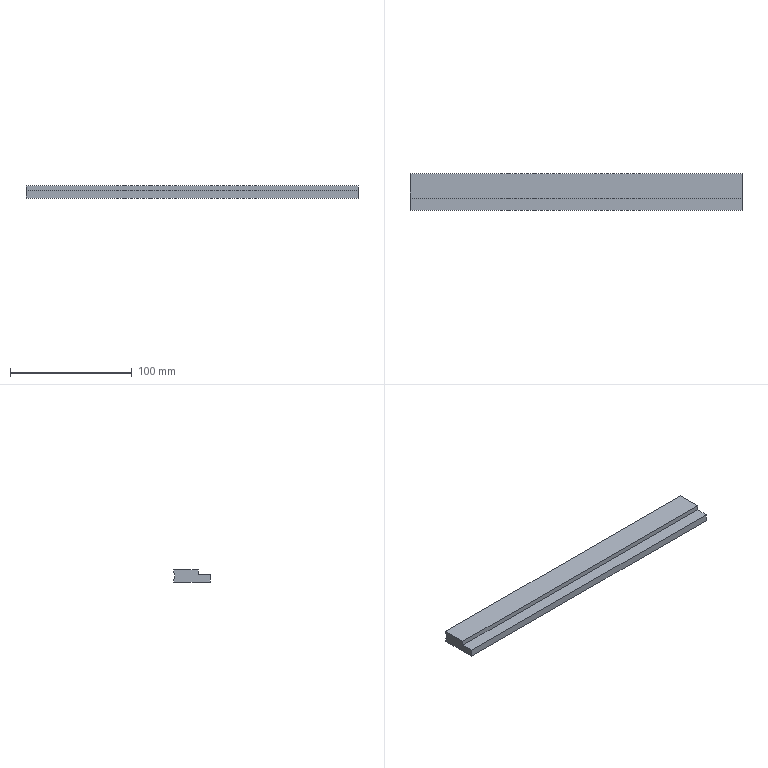Part | STEP file | 001-011-Blanking flip guide rod mounting seat | 1 solid | 10 faces | box 273 x 30 x 10 mm | volume 69990 mm3 | plane 9 | cylinder 1 | commonest cylinder face diameters 8 x1
STEP:
#1=CARTESIAN_POINT('',(0.,0.,0.));
#2=DIRECTION('',(0.,0.,1.));
#3=DIRECTION('',(1.,0.,0.));
#4=AXIS2_PLACEMENT_3D('',#1,#2,#3);
#5=CARTESIAN_POINT('',(-136.5,15.,2.354));
#6=VERTEX_POINT('',#5);
#7=CARTESIAN_POINT('',(-136.5,15.,0.));
#8=VERTEX_POINT('',#7);
#9=CARTESIAN_POINT('',(-136.5,15.,10.));
#10=DIRECTION('',(0.,0.,-1.));
#11=VECTOR('',#10,1.);
#12=LINE('',#9,#11);
#13=CARTESIAN_POINT('',(-136.5,15.,10.));
#14=DIRECTION('',(0.,-1.,0.));
#15=DIRECTION('',(1.,0.,0.));
#16=AXIS2_PLACEMENT_3D('',#13,#14,#15);
#17=PLANE('',#16);
#18=CARTESIAN_POINT('',(0.,0.));
#19=DIRECTION('',(0.,-1.));
#20=VECTOR('',#19,1.);
#21=LINE('',#18,#20);
#22=(GEOMETRIC_REPRESENTATION_CONTEXT(2)PARAMETRIC_REPRESENTATION_CONTEXT()REPRESENTATION_CONTEXT('',''));
#23=DEFINITIONAL_REPRESENTATION('',(#21),#22);
#24=PCURVE('',#17,#23);
#25=CARTESIAN_POINT('',(-136.5,-15.,10.));
#26=DIRECTION('',(1.,0.,0.));
#27=DIRECTION('',(0.,0.,-1.));
#28=AXIS2_PLACEMENT_3D('',#25,#26,#27);
#29=PLANE('',#28);
#30=CARTESIAN_POINT('',(0.,30.));
#31=DIRECTION('',(1.,0.));
#32=VECTOR('',#31,1.);
#33=LINE('',#30,#32);
#34=(GEOMETRIC_REPRESENTATION_CONTEXT(2)PARAMETRIC_REPRESENTATION_CONTEXT()REPRESENTATION_CONTEXT('',''));
#35=DEFINITIONAL_REPRESENTATION('',(#33),#34);
#36=PCURVE('',#29,#35);
#37=SURFACE_CURVE('',#12,(#24,#36),.PCURVE_S1.);
#38=EDGE_CURVE('',#6,#8,#37,.T.);
#39=ORIENTED_EDGE('',*,*,#38,.F.);
#40=CARTESIAN_POINT('',(136.5,15.,2.354));
#41=VERTEX_POINT('',#40);
#42=CARTESIAN_POINT('',(-136.5,15.,2.354));
#43=DIRECTION('',(1.,0.,0.));
#44=VECTOR('',#43,1.);
#45=LINE('',#42,#44);
#46=CARTESIAN_POINT('',(0.,-7.646));
#47=DIRECTION('',(1.,0.));
#48=VECTOR('',#47,1.);
#49=LINE('',#46,#48);
#50=(GEOMETRIC_REPRESENTATION_CONTEXT(2)PARAMETRIC_REPRESENTATION_CONTEXT()REPRESENTATION_CONTEXT('',''));
#51=DEFINITIONAL_REPRESENTATION('',(#49),#50);
#52=PCURVE('',#17,#51);
#53=CARTESIAN_POINT('',(-136.5,18.,5.));
#54=DIRECTION('',(1.,0.,0.));
#55=DIRECTION('',(0.,0.,-1.));
#56=AXIS2_PLACEMENT_3D('',#53,#54,#55);
#57=CYLINDRICAL_SURFACE('',#56,4.);
#58=CARTESIAN_POINT('',(5.435,0.));
#59=DIRECTION('',(0.,1.));
#60=VECTOR('',#59,1.);
#61=LINE('',#58,#60);
#62=(GEOMETRIC_REPRESENTATION_CONTEXT(2)PARAMETRIC_REPRESENTATION_CONTEXT()REPRESENTATION_CONTEXT('',''));
#63=DEFINITIONAL_REPRESENTATION('',(#61),#62);
#64=PCURVE('',#57,#63);
#65=SURFACE_CURVE('',#45,(#52,#64),.PCURVE_S1.);
#66=EDGE_CURVE('',#6,#41,#65,.T.);
#67=ORIENTED_EDGE('',*,*,#66,.T.);
#68=CARTESIAN_POINT('',(136.5,15.,0.));
#69=VERTEX_POINT('',#68);
#70=CARTESIAN_POINT('',(136.5,15.,10.));
#71=DIRECTION('',(0.,0.,-1.));
#72=VECTOR('',#71,1.);
#73=LINE('',#70,#72);
#74=CARTESIAN_POINT('',(273.,0.));
#75=DIRECTION('',(0.,-1.));
#76=VECTOR('',#75,1.);
#77=LINE('',#74,#76);
#78=(GEOMETRIC_REPRESENTATION_CONTEXT(2)PARAMETRIC_REPRESENTATION_CONTEXT()REPRESENTATION_CONTEXT('',''));
#79=DEFINITIONAL_REPRESENTATION('',(#77),#78);
#80=PCURVE('',#17,#79);
#81=CARTESIAN_POINT('',(136.5,-15.,10.));
#82=DIRECTION('',(-1.,0.,0.));
#83=DIRECTION('',(0.,0.,1.));
#84=AXIS2_PLACEMENT_3D('',#81,#82,#83);
#85=PLANE('',#84);
#86=CARTESIAN_POINT('',(0.,30.));
#87=DIRECTION('',(-1.,0.));
#88=VECTOR('',#87,1.);
#89=LINE('',#86,#88);
#90=(GEOMETRIC_REPRESENTATION_CONTEXT(2)PARAMETRIC_REPRESENTATION_CONTEXT()REPRESENTATION_CONTEXT('',''));
#91=DEFINITIONAL_REPRESENTATION('',(#89),#90);
#92=PCURVE('',#85,#91);
#93=SURFACE_CURVE('',#73,(#80,#92),.PCURVE_S1.);
#94=EDGE_CURVE('',#41,#69,#93,.T.);
#95=ORIENTED_EDGE('',*,*,#94,.T.);
#96=CARTESIAN_POINT('',(-136.5,15.,0.));
#97=DIRECTION('',(-1.,0.,0.));
#98=VECTOR('',#97,1.);
#99=LINE('',#96,#98);
#100=CARTESIAN_POINT('',(0.,-10.));
#101=DIRECTION('',(-1.,0.));
#102=VECTOR('',#101,1.);
#103=LINE('',#100,#102);
#104=(GEOMETRIC_REPRESENTATION_CONTEXT(2)PARAMETRIC_REPRESENTATION_CONTEXT()REPRESENTATION_CONTEXT('',''));
#105=DEFINITIONAL_REPRESENTATION('',(#103),#104);
#106=PCURVE('',#17,#105);
#107=CARTESIAN_POINT('',(0.,0.,0.));
#108=DIRECTION('',(0.,0.,-1.));
#109=DIRECTION('',(-1.,0.,0.));
#110=AXIS2_PLACEMENT_3D('',#107,#108,#109);
#111=PLANE('',#110);
#112=CARTESIAN_POINT('',(136.5,15.));
#113=DIRECTION('',(1.,0.));
#114=VECTOR('',#113,1.);
#115=LINE('',#112,#114);
#116=(GEOMETRIC_REPRESENTATION_CONTEXT(2)PARAMETRIC_REPRESENTATION_CONTEXT()REPRESENTATION_CONTEXT('',''));
#117=DEFINITIONAL_REPRESENTATION('',(#115),#116);
#118=PCURVE('',#111,#117);
#119=SURFACE_CURVE('',#99,(#106,#118),.PCURVE_S1.);
#120=EDGE_CURVE('',#69,#8,#119,.T.);
#121=ORIENTED_EDGE('',*,*,#120,.T.);
#122=EDGE_LOOP('',(#39,#67,#95,#121));
#123=FACE_BOUND('',#122,.T.);
#124=ADVANCED_FACE('',(#123),#17,.F.);
#125=CARTESIAN_POINT('',(136.5,-5.,10.));
#126=VERTEX_POINT('',#125);
#127=CARTESIAN_POINT('',(136.5,15.,10.));
#128=VERTEX_POINT('',#127);
#129=CARTESIAN_POINT('',(136.5,-15.,10.));
#130=DIRECTION('',(0.,1.,0.));
#131=VECTOR('',#130,1.);
#132=LINE('',#129,#131);
#133=CARTESIAN_POINT('',(0.,0.));
#134=DIRECTION('',(0.,1.));
#135=VECTOR('',#134,1.);
#136=LINE('',#133,#135);
#137=(GEOMETRIC_REPRESENTATION_CONTEXT(2)PARAMETRIC_REPRESENTATION_CONTEXT()REPRESENTATION_CONTEXT('',''));
#138=DEFINITIONAL_REPRESENTATION('',(#136),#137);
#139=PCURVE('',#85,#138);
#140=CARTESIAN_POINT('',(0.,0.,10.));
#141=DIRECTION('',(0.,0.,-1.));
#142=DIRECTION('',(-1.,0.,0.));
#143=AXIS2_PLACEMENT_3D('',#140,#141,#142);
#144=PLANE('',#143);
#145=CARTESIAN_POINT('',(-136.5,-15.));
#146=DIRECTION('',(0.,1.));
#147=VECTOR('',#146,1.);
#148=LINE('',#145,#147);
#149=(GEOMETRIC_REPRESENTATION_CONTEXT(2)PARAMETRIC_REPRESENTATION_CONTEXT()REPRESENTATION_CONTEXT('',''));
#150=DEFINITIONAL_REPRESENTATION('',(#148),#149);
#151=PCURVE('',#144,#150);
#152=SURFACE_CURVE('',#132,(#139,#151),.PCURVE_S1.);
#153=EDGE_CURVE('',#126,#128,#152,.T.);
#154=ORIENTED_EDGE('',*,*,#153,.F.);
#155=CARTESIAN_POINT('',(136.5,-5.,6.));
#156=VERTEX_POINT('',#155);
#157=CARTESIAN_POINT('',(136.5,-5.,6.));
#158=DIRECTION('',(0.,0.,1.));
#159=VECTOR('',#158,1.);
#160=LINE('',#157,#159);
#161=CARTESIAN_POINT('',(-4.,10.));
#162=DIRECTION('',(1.,0.));
#163=VECTOR('',#162,1.);
#164=LINE('',#161,#163);
#165=(GEOMETRIC_REPRESENTATION_CONTEXT(2)PARAMETRIC_REPRESENTATION_CONTEXT()REPRESENTATION_CONTEXT('',''));
#166=DEFINITIONAL_REPRESENTATION('',(#164),#165);
#167=PCURVE('',#85,#166);
#168=CARTESIAN_POINT('',(-136.5,-5.,6.));
#169=DIRECTION('',(0.,1.,0.));
#170=DIRECTION('',(0.,0.,1.));
#171=AXIS2_PLACEMENT_3D('',#168,#169,#170);
#172=PLANE('',#171);
#173=CARTESIAN_POINT('',(0.,273.));
#174=DIRECTION('',(1.,0.));
#175=VECTOR('',#174,1.);
#176=LINE('',#173,#175);
#177=(GEOMETRIC_REPRESENTATION_CONTEXT(2)PARAMETRIC_REPRESENTATION_CONTEXT()REPRESENTATION_CONTEXT('',''));
#178=DEFINITIONAL_REPRESENTATION('',(#176),#177);
#179=PCURVE('',#172,#178);
#180=SURFACE_CURVE('',#160,(#167,#179),.PCURVE_S1.);
#181=EDGE_CURVE('',#156,#126,#180,.T.);
#182=ORIENTED_EDGE('',*,*,#181,.F.);
#183=CARTESIAN_POINT('',(136.5,-15.,6.));
#184=VERTEX_POINT('',#183);
#185=CARTESIAN_POINT('',(136.5,-15.,6.));
#186=DIRECTION('',(0.,1.,0.));
#187=VECTOR('',#186,1.);
#188=LINE('',#185,#187);
#189=CARTESIAN_POINT('',(-4.,0.));
#190=DIRECTION('',(0.,1.));
#191=VECTOR('',#190,1.);
#192=LINE('',#189,#191);
#193=(GEOMETRIC_REPRESENTATION_CONTEXT(2)PARAMETRIC_REPRESENTATION_CONTEXT()REPRESENTATION_CONTEXT('',''));
#194=DEFINITIONAL_REPRESENTATION('',(#192),#193);
#195=PCURVE('',#85,#194);
#196=CARTESIAN_POINT('',(0.,0.,6.));
#197=DIRECTION('',(0.,0.,-1.));
#198=DIRECTION('',(-1.,0.,0.));
#199=AXIS2_PLACEMENT_3D('',#196,#197,#198);
#200=PLANE('',#199);
#201=CARTESIAN_POINT('',(-136.5,-15.));
#202=DIRECTION('',(0.,1.));
#203=VECTOR('',#202,1.);
#204=LINE('',#201,#203);
#205=(GEOMETRIC_REPRESENTATION_CONTEXT(2)PARAMETRIC_REPRESENTATION_CONTEXT()REPRESENTATION_CONTEXT('',''));
#206=DEFINITIONAL_REPRESENTATION('',(#204),#205);
#207=PCURVE('',#200,#206);
#208=SURFACE_CURVE('',#188,(#195,#207),.PCURVE_S1.);
#209=EDGE_CURVE('',#184,#156,#208,.T.);
#210=ORIENTED_EDGE('',*,*,#209,.F.);
#211=CARTESIAN_POINT('',(136.5,-15.,0.));
#212=VERTEX_POINT('',#211);
#213=CARTESIAN_POINT('',(136.5,-15.,10.));
#214=DIRECTION('',(0.,0.,-1.));
#215=VECTOR('',#214,1.);
#216=LINE('',#213,#215);
#217=CARTESIAN_POINT('',(0.,0.));
#218=DIRECTION('',(-1.,0.));
#219=VECTOR('',#218,1.);
#220=LINE('',#217,#219);
#221=(GEOMETRIC_REPRESENTATION_CONTEXT(2)PARAMETRIC_REPRESENTATION_CONTEXT()REPRESENTATION_CONTEXT('',''));
#222=DEFINITIONAL_REPRESENTATION('',(#220),#221);
#223=PCURVE('',#85,#222);
#224=CARTESIAN_POINT('',(-136.5,-15.,10.));
#225=DIRECTION('',(0.,1.,0.));
#226=DIRECTION('',(-1.,0.,0.));
#227=AXIS2_PLACEMENT_3D('',#224,#225,#226);
#228=PLANE('',#227);
#229=CARTESIAN_POINT('',(-273.,0.));
#230=DIRECTION('',(0.,-1.));
#231=VECTOR('',#230,1.);
#232=LINE('',#229,#231);
#233=(GEOMETRIC_REPRESENTATION_CONTEXT(2)PARAMETRIC_REPRESENTATION_CONTEXT()REPRESENTATION_CONTEXT('',''));
#234=DEFINITIONAL_REPRESENTATION('',(#232),#233);
#235=PCURVE('',#228,#234);
#236=SURFACE_CURVE('',#216,(#223,#235),.PCURVE_S1.);
#237=EDGE_CURVE('',#184,#212,#236,.T.);
#238=ORIENTED_EDGE('',*,*,#237,.T.);
#239=CARTESIAN_POINT('',(136.5,-15.,0.));
#240=DIRECTION('',(0.,1.,0.));
#241=VECTOR('',#240,1.);
#242=LINE('',#239,#241);
#243=CARTESIAN_POINT('',(-10.,0.));
#244=DIRECTION('',(0.,1.));
#245=VECTOR('',#244,1.);
#246=LINE('',#243,#245);
#247=(GEOMETRIC_REPRESENTATION_CONTEXT(2)PARAMETRIC_REPRESENTATION_CONTEXT()REPRESENTATION_CONTEXT('',''));
#248=DEFINITIONAL_REPRESENTATION('',(#246),#247);
#249=PCURVE('',#85,#248);
#250=CARTESIAN_POINT('',(-136.5,-15.));
#251=DIRECTION('',(0.,1.));
#252=VECTOR('',#251,1.);
#253=LINE('',#250,#252);
#254=(GEOMETRIC_REPRESENTATION_CONTEXT(2)PARAMETRIC_REPRESENTATION_CONTEXT()REPRESENTATION_CONTEXT('',''));
#255=DEFINITIONAL_REPRESENTATION('',(#253),#254);
#256=PCURVE('',#111,#255);
#257=SURFACE_CURVE('',#242,(#249,#256),.PCURVE_S1.);
#258=EDGE_CURVE('',#212,#69,#257,.T.);
#259=ORIENTED_EDGE('',*,*,#258,.T.);
#260=ORIENTED_EDGE('',*,*,#94,.F.);
#261=CARTESIAN_POINT('',(136.5,15.,7.646));
#262=VERTEX_POINT('',#261);
#263=CARTESIAN_POINT('',(136.5,18.,5.));
#264=DIRECTION('',(1.,0.,0.));
#265=DIRECTION('',(0.,0.,-1.));
#266=AXIS2_PLACEMENT_3D('',#263,#264,#265);
#267=CIRCLE('',#266,4.);
#268=CARTESIAN_POINT('',(-9.,33.));
#269=CARTESIAN_POINT('',(-9.,39.928));
#270=CARTESIAN_POINT('',(-3.,36.464));
#271=CARTESIAN_POINT('',(3.,33.));
#272=CARTESIAN_POINT('',(-3.,29.536));
#273=CARTESIAN_POINT('',(-9.,26.072));
#274=CARTESIAN_POINT('',(-9.,33.));
#275=(BOUNDED_CURVE()B_SPLINE_CURVE(2,(#268,#269,#270,#271,#272,#273,#274),.UNSPECIFIED.,.T.,.F.)B_SPLINE_CURVE_WITH_KNOTS((1,2,2,2,2,1),(-2.094,0.,2.094,4.189,6.283,8.378),.UNSPECIFIED.)CURVE()GEOMETRIC_REPRESENTATION_ITEM()RATIONAL_B_SPLINE_CURVE((1.,0.5,1.,0.5,1.,0.5,1.))REPRESENTATION_ITEM(''));
#276=(GEOMETRIC_REPRESENTATION_CONTEXT(2)PARAMETRIC_REPRESENTATION_CONTEXT()REPRESENTATION_CONTEXT('',''));
#277=DEFINITIONAL_REPRESENTATION('',(#275),#276);
#278=PCURVE('',#85,#277);
#279=CARTESIAN_POINT('',(0.,273.));
#280=DIRECTION('',(1.,0.));
#281=VECTOR('',#280,1.);
#282=LINE('',#279,#281);
#283=(GEOMETRIC_REPRESENTATION_CONTEXT(2)PARAMETRIC_REPRESENTATION_CONTEXT()REPRESENTATION_CONTEXT('',''));
#284=DEFINITIONAL_REPRESENTATION('',(#282),#283);
#285=PCURVE('',#57,#284);
#286=SURFACE_CURVE('',#267,(#278,#285),.PCURVE_S1.);
#287=EDGE_CURVE('',#262,#41,#286,.T.);
#288=ORIENTED_EDGE('',*,*,#287,.F.);
#289=CARTESIAN_POINT('',(136.5,15.,10.));
#290=DIRECTION('',(0.,0.,-1.));
#291=VECTOR('',#290,1.);
#292=LINE('',#289,#291);
#293=CARTESIAN_POINT('',(0.,30.));
#294=DIRECTION('',(-1.,0.));
#295=VECTOR('',#294,1.);
#296=LINE('',#293,#295);
#297=(GEOMETRIC_REPRESENTATION_CONTEXT(2)PARAMETRIC_REPRESENTATION_CONTEXT()REPRESENTATION_CONTEXT('',''));
#298=DEFINITIONAL_REPRESENTATION('',(#296),#297);
#299=PCURVE('',#85,#298);
#300=CARTESIAN_POINT('',(-136.5,15.,10.));
#301=DIRECTION('',(0.,-1.,0.));
#302=DIRECTION('',(1.,0.,0.));
#303=AXIS2_PLACEMENT_3D('',#300,#301,#302);
#304=PLANE('',#303);
#305=CARTESIAN_POINT('',(273.,0.));
#306=DIRECTION('',(0.,-1.));
#307=VECTOR('',#306,1.);
#308=LINE('',#305,#307);
#309=(GEOMETRIC_REPRESENTATION_CONTEXT(2)PARAMETRIC_REPRESENTATION_CONTEXT()REPRESENTATION_CONTEXT('',''));
#310=DEFINITIONAL_REPRESENTATION('',(#308),#309);
#311=PCURVE('',#304,#310);
#312=SURFACE_CURVE('',#292,(#299,#311),.PCURVE_S1.);
#313=EDGE_CURVE('',#128,#262,#312,.T.);
#314=ORIENTED_EDGE('',*,*,#313,.F.);
#315=EDGE_LOOP('',(#154,#182,#210,#238,#259,#260,#288,#314));
#316=FACE_BOUND('',#315,.T.);
#317=ADVANCED_FACE('',(#316),#85,.F.);
#318=ORIENTED_EDGE('',*,*,#313,.T.);
#319=CARTESIAN_POINT('',(-136.5,15.,7.646));
#320=VERTEX_POINT('',#319);
#321=CARTESIAN_POINT('',(-136.5,15.,7.646));
#322=DIRECTION('',(-1.,0.,0.));
#323=VECTOR('',#322,1.);
#324=LINE('',#321,#323);
#325=CARTESIAN_POINT('',(0.,-2.354));
#326=DIRECTION('',(-1.,0.));
#327=VECTOR('',#326,1.);
#328=LINE('',#325,#327);
#329=(GEOMETRIC_REPRESENTATION_CONTEXT(2)PARAMETRIC_REPRESENTATION_CONTEXT()REPRESENTATION_CONTEXT('',''));
#330=DEFINITIONAL_REPRESENTATION('',(#328),#329);
#331=PCURVE('',#304,#330);
#332=CARTESIAN_POINT('',(3.99,0.));
#333=DIRECTION('',(0.,-1.));
#334=VECTOR('',#333,1.);
#335=LINE('',#332,#334);
#336=(GEOMETRIC_REPRESENTATION_CONTEXT(2)PARAMETRIC_REPRESENTATION_CONTEXT()REPRESENTATION_CONTEXT('',''));
#337=DEFINITIONAL_REPRESENTATION('',(#335),#336);
#338=PCURVE('',#57,#337);
#339=SURFACE_CURVE('',#324,(#331,#338),.PCURVE_S1.);
#340=EDGE_CURVE('',#262,#320,#339,.T.);
#341=ORIENTED_EDGE('',*,*,#340,.T.);
#342=CARTESIAN_POINT('',(-136.5,15.,10.));
#343=VERTEX_POINT('',#342);
#344=CARTESIAN_POINT('',(-136.5,15.,10.));
#345=DIRECTION('',(0.,0.,-1.));
#346=VECTOR('',#345,1.);
#347=LINE('',#344,#346);
#348=CARTESIAN_POINT('',(0.,0.));
#349=DIRECTION('',(0.,-1.));
#350=VECTOR('',#349,1.);
#351=LINE('',#348,#350);
#352=(GEOMETRIC_REPRESENTATION_CONTEXT(2)PARAMETRIC_REPRESENTATION_CONTEXT()REPRESENTATION_CONTEXT('',''));
#353=DEFINITIONAL_REPRESENTATION('',(#351),#352);
#354=PCURVE('',#304,#353);
#355=CARTESIAN_POINT('',(0.,30.));
#356=DIRECTION('',(1.,0.));
#357=VECTOR('',#356,1.);
#358=LINE('',#355,#357);
#359=(GEOMETRIC_REPRESENTATION_CONTEXT(2)PARAMETRIC_REPRESENTATION_CONTEXT()REPRESENTATION_CONTEXT('',''));
#360=DEFINITIONAL_REPRESENTATION('',(#358),#359);
#361=PCURVE('',#29,#360);
#362=SURFACE_CURVE('',#347,(#354,#361),.PCURVE_S1.);
#363=EDGE_CURVE('',#343,#320,#362,.T.);
#364=ORIENTED_EDGE('',*,*,#363,.F.);
#365=CARTESIAN_POINT('',(-136.5,15.,10.));
#366=DIRECTION('',(-1.,0.,0.));
#367=VECTOR('',#366,1.);
#368=LINE('',#365,#367);
#369=CARTESIAN_POINT('',(0.,0.));
#370=DIRECTION('',(-1.,0.));
#371=VECTOR('',#370,1.);
#372=LINE('',#369,#371);
#373=(GEOMETRIC_REPRESENTATION_CONTEXT(2)PARAMETRIC_REPRESENTATION_CONTEXT()REPRESENTATION_CONTEXT('',''));
#374=DEFINITIONAL_REPRESENTATION('',(#372),#373);
#375=PCURVE('',#304,#374);
#376=CARTESIAN_POINT('',(136.5,15.));
#377=DIRECTION('',(1.,0.));
#378=VECTOR('',#377,1.);
#379=LINE('',#376,#378);
#380=(GEOMETRIC_REPRESENTATION_CONTEXT(2)PARAMETRIC_REPRESENTATION_CONTEXT()REPRESENTATION_CONTEXT('',''));
#381=DEFINITIONAL_REPRESENTATION('',(#379),#380);
#382=PCURVE('',#144,#381);
#383=SURFACE_CURVE('',#368,(#375,#382),.PCURVE_S1.);
#384=EDGE_CURVE('',#128,#343,#383,.T.);
#385=ORIENTED_EDGE('',*,*,#384,.F.);
#386=EDGE_LOOP('',(#318,#341,#364,#385));
#387=FACE_BOUND('',#386,.T.);
#388=ADVANCED_FACE('',(#387),#304,.F.);
#389=CARTESIAN_POINT('',(-136.5,-5.,6.));
#390=VERTEX_POINT('',#389);
#391=CARTESIAN_POINT('',(-136.5,-15.,6.));
#392=VERTEX_POINT('',#391);
#393=CARTESIAN_POINT('',(-136.5,-15.,6.));
#394=DIRECTION('',(0.,-1.,0.));
#395=VECTOR('',#394,1.);
#396=LINE('',#393,#395);
#397=CARTESIAN_POINT('',(4.,0.));
#398=DIRECTION('',(0.,-1.));
#399=VECTOR('',#398,1.);
#400=LINE('',#397,#399);
#401=(GEOMETRIC_REPRESENTATION_CONTEXT(2)PARAMETRIC_REPRESENTATION_CONTEXT()REPRESENTATION_CONTEXT('',''));
#402=DEFINITIONAL_REPRESENTATION('',(#400),#401);
#403=PCURVE('',#29,#402);
#404=CARTESIAN_POINT('',(136.5,-15.));
#405=DIRECTION('',(0.,-1.));
#406=VECTOR('',#405,1.);
#407=LINE('',#404,#406);
#408=(GEOMETRIC_REPRESENTATION_CONTEXT(2)PARAMETRIC_REPRESENTATION_CONTEXT()REPRESENTATION_CONTEXT('',''));
#409=DEFINITIONAL_REPRESENTATION('',(#407),#408);
#410=PCURVE('',#200,#409);
#411=SURFACE_CURVE('',#396,(#403,#410),.PCURVE_S1.);
#412=EDGE_CURVE('',#390,#392,#411,.T.);
#413=ORIENTED_EDGE('',*,*,#412,.F.);
#414=CARTESIAN_POINT('',(-136.5,-5.,10.));
#415=VERTEX_POINT('',#414);
#416=CARTESIAN_POINT('',(-136.5,-5.,6.));
#417=DIRECTION('',(0.,0.,1.));
#418=VECTOR('',#417,1.);
#419=LINE('',#416,#418);
#420=CARTESIAN_POINT('',(4.,10.));
#421=DIRECTION('',(-1.,0.));
#422=VECTOR('',#421,1.);
#423=LINE('',#420,#422);
#424=(GEOMETRIC_REPRESENTATION_CONTEXT(2)PARAMETRIC_REPRESENTATION_CONTEXT()REPRESENTATION_CONTEXT('',''));
#425=DEFINITIONAL_REPRESENTATION('',(#423),#424);
#426=PCURVE('',#29,#425);
#427=CARTESIAN_POINT('',(0.,0.));
#428=DIRECTION('',(1.,0.));
#429=VECTOR('',#428,1.);
#430=LINE('',#427,#429);
#431=(GEOMETRIC_REPRESENTATION_CONTEXT(2)PARAMETRIC_REPRESENTATION_CONTEXT()REPRESENTATION_CONTEXT('',''));
#432=DEFINITIONAL_REPRESENTATION('',(#430),#431);
#433=PCURVE('',#172,#432);
#434=SURFACE_CURVE('',#419,(#426,#433),.PCURVE_S1.);
#435=EDGE_CURVE('',#390,#415,#434,.T.);
#436=ORIENTED_EDGE('',*,*,#435,.T.);
#437=CARTESIAN_POINT('',(-136.5,-15.,10.));
#438=DIRECTION('',(0.,-1.,0.));
#439=VECTOR('',#438,1.);
#440=LINE('',#437,#439);
#441=CARTESIAN_POINT('',(0.,0.));
#442=DIRECTION('',(0.,-1.));
#443=VECTOR('',#442,1.);
#444=LINE('',#441,#443);
#445=(GEOMETRIC_REPRESENTATION_CONTEXT(2)PARAMETRIC_REPRESENTATION_CONTEXT()REPRESENTATION_CONTEXT('',''));
#446=DEFINITIONAL_REPRESENTATION('',(#444),#445);
#447=PCURVE('',#29,#446);
#448=CARTESIAN_POINT('',(136.5,-15.));
#449=DIRECTION('',(0.,-1.));
#450=VECTOR('',#449,1.);
#451=LINE('',#448,#450);
#452=(GEOMETRIC_REPRESENTATION_CONTEXT(2)PARAMETRIC_REPRESENTATION_CONTEXT()REPRESENTATION_CONTEXT('',''));
#453=DEFINITIONAL_REPRESENTATION('',(#451),#452);
#454=PCURVE('',#144,#453);
#455=SURFACE_CURVE('',#440,(#447,#454),.PCURVE_S1.);
#456=EDGE_CURVE('',#343,#415,#455,.T.);
#457=ORIENTED_EDGE('',*,*,#456,.F.);
#458=ORIENTED_EDGE('',*,*,#363,.T.);
#459=CARTESIAN_POINT('',(-136.5,18.,5.));
#460=DIRECTION('',(1.,0.,0.));
#461=DIRECTION('',(0.,0.,-1.));
#462=AXIS2_PLACEMENT_3D('',#459,#460,#461);
#463=CIRCLE('',#462,4.);
#464=CARTESIAN_POINT('',(5.,33.));
#465=DIRECTION('',(1.,0.));
#466=AXIS2_PLACEMENT_2D('',#464,#465);
#467=CIRCLE('',#466,4.);
#468=(GEOMETRIC_REPRESENTATION_CONTEXT(2)PARAMETRIC_REPRESENTATION_CONTEXT()REPRESENTATION_CONTEXT('',''));
#469=DEFINITIONAL_REPRESENTATION('',(#467),#468);
#470=PCURVE('',#29,#469);
#471=CARTESIAN_POINT('',(0.,0.));
#472=DIRECTION('',(1.,0.));
#473=VECTOR('',#472,1.);
#474=LINE('',#471,#473);
#475=(GEOMETRIC_REPRESENTATION_CONTEXT(2)PARAMETRIC_REPRESENTATION_CONTEXT()REPRESENTATION_CONTEXT('',''));
#476=DEFINITIONAL_REPRESENTATION('',(#474),#475);
#477=PCURVE('',#57,#476);
#478=SURFACE_CURVE('',#463,(#470,#477),.PCURVE_S1.);
#479=EDGE_CURVE('',#320,#6,#478,.T.);
#480=ORIENTED_EDGE('',*,*,#479,.T.);
#481=ORIENTED_EDGE('',*,*,#38,.T.);
#482=CARTESIAN_POINT('',(-136.5,-15.,0.));
#483=VERTEX_POINT('',#482);
#484=CARTESIAN_POINT('',(-136.5,-15.,0.));
#485=DIRECTION('',(0.,-1.,0.));
#486=VECTOR('',#485,1.);
#487=LINE('',#484,#486);
#488=CARTESIAN_POINT('',(10.,0.));
#489=DIRECTION('',(0.,-1.));
#490=VECTOR('',#489,1.);
#491=LINE('',#488,#490);
#492=(GEOMETRIC_REPRESENTATION_CONTEXT(2)PARAMETRIC_REPRESENTATION_CONTEXT()REPRESENTATION_CONTEXT('',''));
#493=DEFINITIONAL_REPRESENTATION('',(#491),#492);
#494=PCURVE('',#29,#493);
#495=CARTESIAN_POINT('',(136.5,-15.));
#496=DIRECTION('',(0.,-1.));
#497=VECTOR('',#496,1.);
#498=LINE('',#495,#497);
#499=(GEOMETRIC_REPRESENTATION_CONTEXT(2)PARAMETRIC_REPRESENTATION_CONTEXT()REPRESENTATION_CONTEXT('',''));
#500=DEFINITIONAL_REPRESENTATION('',(#498),#499);
#501=PCURVE('',#111,#500);
#502=SURFACE_CURVE('',#487,(#494,#501),.PCURVE_S1.);
#503=EDGE_CURVE('',#8,#483,#502,.T.);
#504=ORIENTED_EDGE('',*,*,#503,.T.);
#505=CARTESIAN_POINT('',(-136.5,-15.,10.));
#506=DIRECTION('',(0.,0.,-1.));
#507=VECTOR('',#506,1.);
#508=LINE('',#505,#507);
#509=CARTESIAN_POINT('',(0.,0.));
#510=DIRECTION('',(1.,0.));
#511=VECTOR('',#510,1.);
#512=LINE('',#509,#511);
#513=(GEOMETRIC_REPRESENTATION_CONTEXT(2)PARAMETRIC_REPRESENTATION_CONTEXT()REPRESENTATION_CONTEXT('',''));
#514=DEFINITIONAL_REPRESENTATION('',(#512),#513);
#515=PCURVE('',#29,#514);
#516=CARTESIAN_POINT('',(0.,0.));
#517=DIRECTION('',(0.,-1.));
#518=VECTOR('',#517,1.);
#519=LINE('',#516,#518);
#520=(GEOMETRIC_REPRESENTATION_CONTEXT(2)PARAMETRIC_REPRESENTATION_CONTEXT()REPRESENTATION_CONTEXT('',''));
#521=DEFINITIONAL_REPRESENTATION('',(#519),#520);
#522=PCURVE('',#228,#521);
#523=SURFACE_CURVE('',#508,(#515,#522),.PCURVE_S1.);
#524=EDGE_CURVE('',#392,#483,#523,.T.);
#525=ORIENTED_EDGE('',*,*,#524,.F.);
#526=EDGE_LOOP('',(#413,#436,#457,#458,#480,#481,#504,#525));
#527=FACE_BOUND('',#526,.T.);
#528=ADVANCED_FACE('',(#527),#29,.F.);
#529=ORIENTED_EDGE('',*,*,#237,.F.);
#530=CARTESIAN_POINT('',(-136.5,-15.,6.));
#531=DIRECTION('',(1.,0.,0.));
#532=VECTOR('',#531,1.);
#533=LINE('',#530,#532);
#534=CARTESIAN_POINT('',(0.,-4.));
#535=DIRECTION('',(-1.,0.));
#536=VECTOR('',#535,1.);
#537=LINE('',#534,#536);
#538=(GEOMETRIC_REPRESENTATION_CONTEXT(2)PARAMETRIC_REPRESENTATION_CONTEXT()REPRESENTATION_CONTEXT('',''));
#539=DEFINITIONAL_REPRESENTATION('',(#537),#538);
#540=PCURVE('',#228,#539);
#541=CARTESIAN_POINT('',(136.5,-15.));
#542=DIRECTION('',(-1.,0.));
#543=VECTOR('',#542,1.);
#544=LINE('',#541,#543);
#545=(GEOMETRIC_REPRESENTATION_CONTEXT(2)PARAMETRIC_REPRESENTATION_CONTEXT()REPRESENTATION_CONTEXT('',''));
#546=DEFINITIONAL_REPRESENTATION('',(#544),#545);
#547=PCURVE('',#200,#546);
#548=SURFACE_CURVE('',#533,(#540,#547),.PCURVE_S1.);
#549=EDGE_CURVE('',#392,#184,#548,.T.);
#550=ORIENTED_EDGE('',*,*,#549,.F.);
#551=ORIENTED_EDGE('',*,*,#524,.T.);
#552=CARTESIAN_POINT('',(-136.5,-15.,0.));
#553=DIRECTION('',(1.,0.,0.));
#554=VECTOR('',#553,1.);
#555=LINE('',#552,#554);
#556=CARTESIAN_POINT('',(0.,-10.));
#557=DIRECTION('',(-1.,0.));
#558=VECTOR('',#557,1.);
#559=LINE('',#556,#558);
#560=(GEOMETRIC_REPRESENTATION_CONTEXT(2)PARAMETRIC_REPRESENTATION_CONTEXT()REPRESENTATION_CONTEXT('',''));
#561=DEFINITIONAL_REPRESENTATION('',(#559),#560);
#562=PCURVE('',#228,#561);
#563=CARTESIAN_POINT('',(136.5,-15.));
#564=DIRECTION('',(-1.,0.));
#565=VECTOR('',#564,1.);
#566=LINE('',#563,#565);
#567=(GEOMETRIC_REPRESENTATION_CONTEXT(2)PARAMETRIC_REPRESENTATION_CONTEXT()REPRESENTATION_CONTEXT('',''));
#568=DEFINITIONAL_REPRESENTATION('',(#566),#567);
#569=PCURVE('',#111,#568);
#570=SURFACE_CURVE('',#555,(#562,#569),.PCURVE_S1.);
#571=EDGE_CURVE('',#483,#212,#570,.T.);
#572=ORIENTED_EDGE('',*,*,#571,.T.);
#573=EDGE_LOOP('',(#529,#550,#551,#572));
#574=FACE_BOUND('',#573,.T.);
#575=ADVANCED_FACE('',(#574),#228,.F.);
#576=ORIENTED_EDGE('',*,*,#456,.T.);
#577=CARTESIAN_POINT('',(-136.5,-5.,10.));
#578=DIRECTION('',(-1.,0.,0.));
#579=VECTOR('',#578,1.);
#580=LINE('',#577,#579);
#581=CARTESIAN_POINT('',(136.5,-5.));
#582=DIRECTION('',(1.,0.));
#583=VECTOR('',#582,1.);
#584=LINE('',#581,#583);
#585=(GEOMETRIC_REPRESENTATION_CONTEXT(2)PARAMETRIC_REPRESENTATION_CONTEXT()REPRESENTATION_CONTEXT('',''));
#586=DEFINITIONAL_REPRESENTATION('',(#584),#585);
#587=PCURVE('',#144,#586);
#588=CARTESIAN_POINT('',(4.,0.));
#589=DIRECTION('',(0.,-1.));
#590=VECTOR('',#589,1.);
#591=LINE('',#588,#590);
#592=(GEOMETRIC_REPRESENTATION_CONTEXT(2)PARAMETRIC_REPRESENTATION_CONTEXT()REPRESENTATION_CONTEXT('',''));
#593=DEFINITIONAL_REPRESENTATION('',(#591),#592);
#594=PCURVE('',#172,#593);
#595=SURFACE_CURVE('',#580,(#587,#594),.PCURVE_S1.);
#596=EDGE_CURVE('',#126,#415,#595,.T.);
#597=ORIENTED_EDGE('',*,*,#596,.F.);
#598=ORIENTED_EDGE('',*,*,#153,.T.);
#599=ORIENTED_EDGE('',*,*,#384,.T.);
#600=EDGE_LOOP('',(#576,#597,#598,#599));
#601=FACE_BOUND('',#600,.T.);
#602=ADVANCED_FACE('',(#601),#144,.F.);
#603=ORIENTED_EDGE('',*,*,#258,.F.);
#604=ORIENTED_EDGE('',*,*,#571,.F.);
#605=ORIENTED_EDGE('',*,*,#503,.F.);
#606=ORIENTED_EDGE('',*,*,#120,.F.);
#607=EDGE_LOOP('',(#603,#604,#605,#606));
#608=FACE_BOUND('',#607,.T.);
#609=ADVANCED_FACE('',(#608),#111,.T.);
#610=ORIENTED_EDGE('',*,*,#66,.T.);
#611=ORIENTED_EDGE('',*,*,#287,.F.);
#612=ORIENTED_EDGE('',*,*,#340,.T.);
#613=ORIENTED_EDGE('',*,*,#479,.T.);
#614=EDGE_LOOP('',(#610,#611,#612,#613));
#615=FACE_BOUND('',#614,.F.);
#616=ADVANCED_FACE('',(#615),#57,.F.);
#617=ORIENTED_EDGE('',*,*,#596,.T.);
#618=ORIENTED_EDGE('',*,*,#435,.F.);
#619=CARTESIAN_POINT('',(-136.5,-5.,6.));
#620=DIRECTION('',(-1.,0.,0.));
#621=VECTOR('',#620,1.);
#622=LINE('',#619,#621);
#623=CARTESIAN_POINT('',(0.,0.));
#624=DIRECTION('',(0.,-1.));
#625=VECTOR('',#624,1.);
#626=LINE('',#623,#625);
#627=(GEOMETRIC_REPRESENTATION_CONTEXT(2)PARAMETRIC_REPRESENTATION_CONTEXT()REPRESENTATION_CONTEXT('',''));
#628=DEFINITIONAL_REPRESENTATION('',(#626),#627);
#629=PCURVE('',#172,#628);
#630=CARTESIAN_POINT('',(136.5,-5.));
#631=DIRECTION('',(1.,0.));
#632=VECTOR('',#631,1.);
#633=LINE('',#630,#632);
#634=(GEOMETRIC_REPRESENTATION_CONTEXT(2)PARAMETRIC_REPRESENTATION_CONTEXT()REPRESENTATION_CONTEXT('',''));
#635=DEFINITIONAL_REPRESENTATION('',(#633),#634);
#636=PCURVE('',#200,#635);
#637=SURFACE_CURVE('',#622,(#629,#636),.PCURVE_S1.);
#638=EDGE_CURVE('',#156,#390,#637,.T.);
#639=ORIENTED_EDGE('',*,*,#638,.F.);
#640=ORIENTED_EDGE('',*,*,#181,.T.);
#641=EDGE_LOOP('',(#617,#618,#639,#640));
#642=FACE_BOUND('',#641,.T.);
#643=ADVANCED_FACE('',(#642),#172,.F.);
#644=ORIENTED_EDGE('',*,*,#412,.T.);
#645=ORIENTED_EDGE('',*,*,#549,.T.);
#646=ORIENTED_EDGE('',*,*,#209,.T.);
#647=ORIENTED_EDGE('',*,*,#638,.T.);
#648=EDGE_LOOP('',(#644,#645,#646,#647));
#649=FACE_BOUND('',#648,.T.);
#650=ADVANCED_FACE('',(#649),#200,.F.);
#651=CLOSED_SHELL('',(#124,#317,#388,#528,#575,#602,#609,#616,#643,#650));
#652=MANIFOLD_SOLID_BREP('',#651);
#653=(LENGTH_UNIT()NAMED_UNIT(*)SI_UNIT(.MILLI.,.METRE.));
#654=UNCERTAINTY_MEASURE_WITH_UNIT(LENGTH_MEASURE(0.0000001),#653,'','');
#655=(NAMED_UNIT(*)PLANE_ANGLE_UNIT()SI_UNIT($,.RADIAN.));
#656=(NAMED_UNIT(*)SI_UNIT($,.STERADIAN.)SOLID_ANGLE_UNIT());
#657=(GEOMETRIC_REPRESENTATION_CONTEXT(3)GLOBAL_UNCERTAINTY_ASSIGNED_CONTEXT((#654))GLOBAL_UNIT_ASSIGNED_CONTEXT((#653,#655,#656))REPRESENTATION_CONTEXT('',''));
#658=ADVANCED_BREP_SHAPE_REPRESENTATION('',(#4,#652),#657);